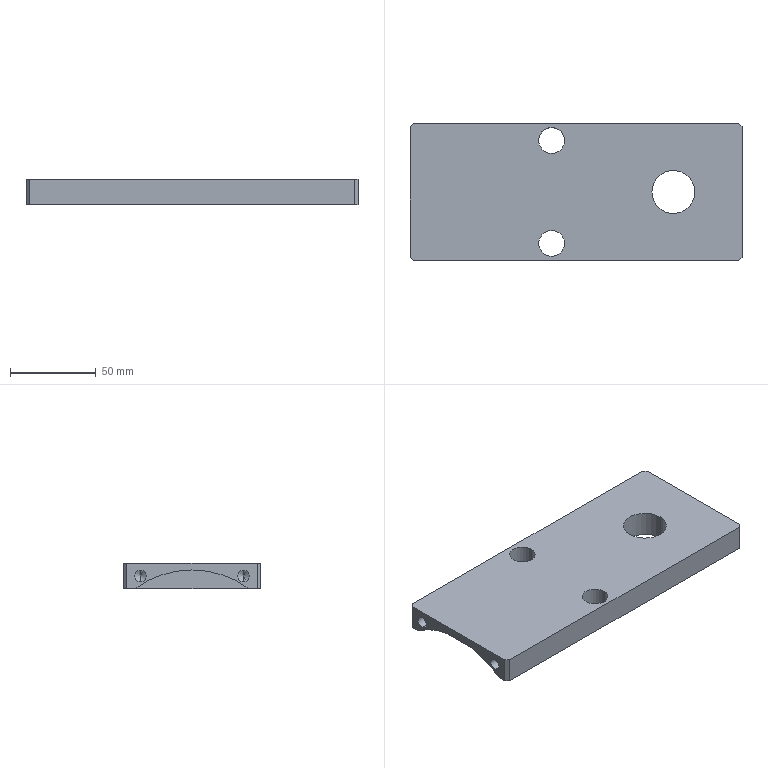Part | SolidWorks | features HoleWzd 4, Chamfer 1, Extrusion 1, ICE 1 | 1 solid | 34 faces | box 193.5 x 80 x 15 mm | volume 211454 mm3 | cylinder 15 | plane 11 | cone 8 | commonest cylinder face diameters 6.8 x8 15 x4 25 x2 112 x1
STEP:
#1=CARTESIAN_POINT('',(-77.,30.,-3.4));
#2=VERTEX_POINT('',#1);
#3=CARTESIAN_POINT('',(-77.,30.,3.4));
#4=VERTEX_POINT('',#3);
#5=CARTESIAN_POINT('',(-77.,30.,0.));
#6=DIRECTION('',(-1.,0.,0.));
#7=DIRECTION('',(0.,0.,1.));
#8=AXIS2_PLACEMENT_3D('',#5,#6,#7);
#9=CIRCLE('',#8,3.4);
#10=EDGE_CURVE('',#2,#4,#9,.T.);
#11=ORIENTED_EDGE('',*,*,#10,.F.);
#12=CARTESIAN_POINT('',(-96.75,30.,-3.4));
#13=VERTEX_POINT('',#12);
#14=CARTESIAN_POINT('',(-96.75,30.,-3.4));
#15=DIRECTION('',(-1.,0.,0.));
#16=VECTOR('',#15,1000.);
#17=LINE('',#14,#16);
#18=EDGE_CURVE('',#2,#13,#17,.T.);
#19=ORIENTED_EDGE('',*,*,#18,.T.);
#20=CARTESIAN_POINT('',(-96.75,30.,3.4));
#21=VERTEX_POINT('',#20);
#22=CARTESIAN_POINT('',(-96.75,30.,0.));
#23=DIRECTION('',(-1.,0.,0.));
#24=DIRECTION('',(0.,0.,1.));
#25=AXIS2_PLACEMENT_3D('',#22,#23,#24);
#26=CIRCLE('',#25,3.4);
#27=EDGE_CURVE('',#13,#21,#26,.T.);
#28=ORIENTED_EDGE('',*,*,#27,.T.);
#29=CARTESIAN_POINT('',(-96.75,30.,3.4));
#30=DIRECTION('',(-1.,0.,0.));
#31=VECTOR('',#30,1000.);
#32=LINE('',#29,#31);
#33=EDGE_CURVE('',#4,#21,#32,.T.);
#34=ORIENTED_EDGE('',*,*,#33,.F.);
#35=EDGE_LOOP('',(#11,#19,#28,#34));
#36=FACE_OUTER_BOUND('',#35,.T.);
#37=CARTESIAN_POINT('',(-96.75,30.,0.));
#38=DIRECTION('',(-1.,0.,0.));
#39=DIRECTION('',(0.,0.,1.));
#40=AXIS2_PLACEMENT_3D('',#37,#38,#39);
#41=CYLINDRICAL_SURFACE('',#40,3.4);
#42=ADVANCED_FACE('',(#36),#41,.F.);
#43=CARTESIAN_POINT('',(-74.957,30.,0.));
#44=VERTEX_POINT('',#43);
#45=CARTESIAN_POINT('',(-77.,30.,3.4));
#46=DIRECTION('',(-0.515,0.,0.8572));
#47=VECTOR('',#46,1000.);
#48=LINE('',#45,#47);
#49=EDGE_CURVE('',#44,#4,#48,.T.);
#50=ORIENTED_EDGE('',*,*,#49,.F.);
#51=CARTESIAN_POINT('',(-77.,30.,-3.4));
#52=DIRECTION('',(-0.515,0.,-0.8572));
#53=VECTOR('',#52,1000.);
#54=LINE('',#51,#53);
#55=EDGE_CURVE('',#44,#2,#54,.T.);
#56=ORIENTED_EDGE('',*,*,#55,.T.);
#57=ORIENTED_EDGE('',*,*,#10,.T.);
#58=EDGE_LOOP('',(#50,#56,#57));
#59=FACE_OUTER_BOUND('',#58,.T.);
#60=CARTESIAN_POINT('',(-77.,30.,0.));
#61=DIRECTION('',(-1.,0.,0.));
#62=DIRECTION('',(0.,0.,1.));
#63=AXIS2_PLACEMENT_3D('',#60,#61,#62);
#64=CONICAL_SURFACE('',#63,3.4,1.03);
#65=ADVANCED_FACE('',(#59),#64,.F.);
#66=CARTESIAN_POINT('',(-77.,-30.,-3.4));
#67=VERTEX_POINT('',#66);
#68=CARTESIAN_POINT('',(-77.,-30.,3.4));
#69=VERTEX_POINT('',#68);
#70=CARTESIAN_POINT('',(-77.,-30.,0.));
#71=DIRECTION('',(-1.,0.,0.));
#72=DIRECTION('',(0.,0.,1.));
#73=AXIS2_PLACEMENT_3D('',#70,#71,#72);
#74=CIRCLE('',#73,3.4);
#75=EDGE_CURVE('',#67,#69,#74,.T.);
#76=ORIENTED_EDGE('',*,*,#75,.F.);
#77=CARTESIAN_POINT('',(-96.75,-30.,-3.4));
#78=VERTEX_POINT('',#77);
#79=CARTESIAN_POINT('',(-96.75,-30.,-3.4));
#80=DIRECTION('',(-1.,0.,0.));
#81=VECTOR('',#80,1000.);
#82=LINE('',#79,#81);
#83=EDGE_CURVE('',#67,#78,#82,.T.);
#84=ORIENTED_EDGE('',*,*,#83,.T.);
#85=CARTESIAN_POINT('',(-96.75,-30.,3.4));
#86=VERTEX_POINT('',#85);
#87=CARTESIAN_POINT('',(-96.75,-30.,0.));
#88=DIRECTION('',(-1.,0.,0.));
#89=DIRECTION('',(0.,0.,1.));
#90=AXIS2_PLACEMENT_3D('',#87,#88,#89);
#91=CIRCLE('',#90,3.4);
#92=EDGE_CURVE('',#78,#86,#91,.T.);
#93=ORIENTED_EDGE('',*,*,#92,.T.);
#94=CARTESIAN_POINT('',(-96.75,-30.,3.4));
#95=DIRECTION('',(-1.,0.,0.));
#96=VECTOR('',#95,1000.);
#97=LINE('',#94,#96);
#98=EDGE_CURVE('',#69,#86,#97,.T.);
#99=ORIENTED_EDGE('',*,*,#98,.F.);
#100=EDGE_LOOP('',(#76,#84,#93,#99));
#101=FACE_OUTER_BOUND('',#100,.T.);
#102=CARTESIAN_POINT('',(-96.75,-30.,0.));
#103=DIRECTION('',(-1.,0.,0.));
#104=DIRECTION('',(0.,0.,1.));
#105=AXIS2_PLACEMENT_3D('',#102,#103,#104);
#106=CYLINDRICAL_SURFACE('',#105,3.4);
#107=ADVANCED_FACE('',(#101),#106,.F.);
#108=CARTESIAN_POINT('',(-74.957,-30.,0.));
#109=VERTEX_POINT('',#108);
#110=CARTESIAN_POINT('',(-77.,-30.,3.4));
#111=DIRECTION('',(-0.515,0.,0.8572));
#112=VECTOR('',#111,1000.);
#113=LINE('',#110,#112);
#114=EDGE_CURVE('',#109,#69,#113,.T.);
#115=ORIENTED_EDGE('',*,*,#114,.F.);
#116=CARTESIAN_POINT('',(-77.,-30.,-3.4));
#117=DIRECTION('',(-0.515,0.,-0.8572));
#118=VECTOR('',#117,1000.);
#119=LINE('',#116,#118);
#120=EDGE_CURVE('',#109,#67,#119,.T.);
#121=ORIENTED_EDGE('',*,*,#120,.T.);
#122=ORIENTED_EDGE('',*,*,#75,.T.);
#123=EDGE_LOOP('',(#115,#121,#122));
#124=FACE_OUTER_BOUND('',#123,.T.);
#125=CARTESIAN_POINT('',(-77.,-30.,0.));
#126=DIRECTION('',(-1.,0.,0.));
#127=DIRECTION('',(0.,0.,1.));
#128=AXIS2_PLACEMENT_3D('',#125,#126,#127);
#129=CONICAL_SURFACE('',#128,3.4,1.03);
#130=ADVANCED_FACE('',(#124),#129,.F.);
#131=CARTESIAN_POINT('',(77.,30.,3.4));
#132=VERTEX_POINT('',#131);
#133=CARTESIAN_POINT('',(77.,30.,-3.4));
#134=VERTEX_POINT('',#133);
#135=CARTESIAN_POINT('',(77.,30.,0.));
#136=DIRECTION('',(1.,0.,0.));
#137=DIRECTION('',(0.,0.,-1.));
#138=AXIS2_PLACEMENT_3D('',#135,#136,#137);
#139=CIRCLE('',#138,3.4);
#140=EDGE_CURVE('',#132,#134,#139,.T.);
#141=ORIENTED_EDGE('',*,*,#140,.F.);
#142=CARTESIAN_POINT('',(96.75,30.,3.4));
#143=VERTEX_POINT('',#142);
#144=CARTESIAN_POINT('',(96.75,30.,3.4));
#145=DIRECTION('',(1.,0.,0.));
#146=VECTOR('',#145,1000.);
#147=LINE('',#144,#146);
#148=EDGE_CURVE('',#132,#143,#147,.T.);
#149=ORIENTED_EDGE('',*,*,#148,.T.);
#150=CARTESIAN_POINT('',(96.75,30.,-3.4));
#151=VERTEX_POINT('',#150);
#152=CARTESIAN_POINT('',(96.75,30.,0.));
#153=DIRECTION('',(1.,0.,0.));
#154=DIRECTION('',(0.,0.,-1.));
#155=AXIS2_PLACEMENT_3D('',#152,#153,#154);
#156=CIRCLE('',#155,3.4);
#157=EDGE_CURVE('',#143,#151,#156,.T.);
#158=ORIENTED_EDGE('',*,*,#157,.T.);
#159=CARTESIAN_POINT('',(96.75,30.,-3.4));
#160=DIRECTION('',(1.,0.,0.));
#161=VECTOR('',#160,1000.);
#162=LINE('',#159,#161);
#163=EDGE_CURVE('',#134,#151,#162,.T.);
#164=ORIENTED_EDGE('',*,*,#163,.F.);
#165=EDGE_LOOP('',(#141,#149,#158,#164));
#166=FACE_OUTER_BOUND('',#165,.T.);
#167=CARTESIAN_POINT('',(96.75,30.,0.));
#168=DIRECTION('',(1.,0.,0.));
#169=DIRECTION('',(0.,0.,-1.));
#170=AXIS2_PLACEMENT_3D('',#167,#168,#169);
#171=CYLINDRICAL_SURFACE('',#170,3.4);
#172=ADVANCED_FACE('',(#166),#171,.F.);
#173=CARTESIAN_POINT('',(74.957,30.,0.));
#174=VERTEX_POINT('',#173);
#175=CARTESIAN_POINT('',(77.,30.,-3.4));
#176=DIRECTION('',(0.515,0.,-0.8572));
#177=VECTOR('',#176,1000.);
#178=LINE('',#175,#177);
#179=EDGE_CURVE('',#174,#134,#178,.T.);
#180=ORIENTED_EDGE('',*,*,#179,.F.);
#181=CARTESIAN_POINT('',(77.,30.,3.4));
#182=DIRECTION('',(0.515,0.,0.8572));
#183=VECTOR('',#182,1000.);
#184=LINE('',#181,#183);
#185=EDGE_CURVE('',#174,#132,#184,.T.);
#186=ORIENTED_EDGE('',*,*,#185,.T.);
#187=ORIENTED_EDGE('',*,*,#140,.T.);
#188=EDGE_LOOP('',(#180,#186,#187));
#189=FACE_OUTER_BOUND('',#188,.T.);
#190=CARTESIAN_POINT('',(77.,30.,0.));
#191=DIRECTION('',(1.,0.,0.));
#192=DIRECTION('',(0.,0.,-1.));
#193=AXIS2_PLACEMENT_3D('',#190,#191,#192);
#194=CONICAL_SURFACE('',#193,3.4,1.03);
#195=ADVANCED_FACE('',(#189),#194,.F.);
#196=CARTESIAN_POINT('',(77.,-30.,3.4));
#197=VERTEX_POINT('',#196);
#198=CARTESIAN_POINT('',(77.,-30.,-3.4));
#199=VERTEX_POINT('',#198);
#200=CARTESIAN_POINT('',(77.,-30.,0.));
#201=DIRECTION('',(1.,0.,0.));
#202=DIRECTION('',(0.,0.,-1.));
#203=AXIS2_PLACEMENT_3D('',#200,#201,#202);
#204=CIRCLE('',#203,3.4);
#205=EDGE_CURVE('',#197,#199,#204,.T.);
#206=ORIENTED_EDGE('',*,*,#205,.F.);
#207=CARTESIAN_POINT('',(96.75,-30.,3.4));
#208=VERTEX_POINT('',#207);
#209=CARTESIAN_POINT('',(96.75,-30.,3.4));
#210=DIRECTION('',(1.,0.,0.));
#211=VECTOR('',#210,1000.);
#212=LINE('',#209,#211);
#213=EDGE_CURVE('',#197,#208,#212,.T.);
#214=ORIENTED_EDGE('',*,*,#213,.T.);
#215=CARTESIAN_POINT('',(96.75,-30.,-3.4));
#216=VERTEX_POINT('',#215);
#217=CARTESIAN_POINT('',(96.75,-30.,0.));
#218=DIRECTION('',(1.,0.,0.));
#219=DIRECTION('',(0.,0.,-1.));
#220=AXIS2_PLACEMENT_3D('',#217,#218,#219);
#221=CIRCLE('',#220,3.4);
#222=EDGE_CURVE('',#208,#216,#221,.T.);
#223=ORIENTED_EDGE('',*,*,#222,.T.);
#224=CARTESIAN_POINT('',(96.75,-30.,-3.4));
#225=DIRECTION('',(1.,0.,0.));
#226=VECTOR('',#225,1000.);
#227=LINE('',#224,#226);
#228=EDGE_CURVE('',#199,#216,#227,.T.);
#229=ORIENTED_EDGE('',*,*,#228,.F.);
#230=EDGE_LOOP('',(#206,#214,#223,#229));
#231=FACE_OUTER_BOUND('',#230,.T.);
#232=CARTESIAN_POINT('',(96.75,-30.,0.));
#233=DIRECTION('',(1.,0.,0.));
#234=DIRECTION('',(0.,0.,-1.));
#235=AXIS2_PLACEMENT_3D('',#232,#233,#234);
#236=CYLINDRICAL_SURFACE('',#235,3.4);
#237=ADVANCED_FACE('',(#231),#236,.F.);
#238=CARTESIAN_POINT('',(74.957,-30.,0.));
#239=VERTEX_POINT('',#238);
#240=CARTESIAN_POINT('',(77.,-30.,-3.4));
#241=DIRECTION('',(0.515,0.,-0.8572));
#242=VECTOR('',#241,1000.);
#243=LINE('',#240,#242);
#244=EDGE_CURVE('',#239,#199,#243,.T.);
#245=ORIENTED_EDGE('',*,*,#244,.F.);
#246=CARTESIAN_POINT('',(77.,-30.,3.4));
#247=DIRECTION('',(0.515,0.,0.8572));
#248=VECTOR('',#247,1000.);
#249=LINE('',#246,#248);
#250=EDGE_CURVE('',#239,#197,#249,.T.);
#251=ORIENTED_EDGE('',*,*,#250,.T.);
#252=ORIENTED_EDGE('',*,*,#205,.T.);
#253=EDGE_LOOP('',(#245,#251,#252));
#254=FACE_OUTER_BOUND('',#253,.T.);
#255=CARTESIAN_POINT('',(77.,-30.,0.));
#256=DIRECTION('',(1.,0.,0.));
#257=DIRECTION('',(0.,0.,-1.));
#258=AXIS2_PLACEMENT_3D('',#255,#256,#257);
#259=CONICAL_SURFACE('',#258,3.4,1.03);
#260=ADVANCED_FACE('',(#254),#259,.F.);
#261=CARTESIAN_POINT('',(-21.75,30.,-7.5));
#262=VERTEX_POINT('',#261);
#263=CARTESIAN_POINT('',(-6.75,30.,-7.5));
#264=VERTEX_POINT('',#263);
#265=CARTESIAN_POINT('',(-14.25,30.,-7.5));
#266=DIRECTION('',(0.,0.,1.));
#267=DIRECTION('',(1.,0.,0.));
#268=AXIS2_PLACEMENT_3D('',#265,#266,#267);
#269=CIRCLE('',#268,7.5);
#270=EDGE_CURVE('',#262,#264,#269,.T.);
#271=ORIENTED_EDGE('',*,*,#270,.F.);
#272=CARTESIAN_POINT('',(-21.75,30.,7.5));
#273=VERTEX_POINT('',#272);
#274=CARTESIAN_POINT('',(-21.75,30.,7.5));
#275=DIRECTION('',(0.,0.,1.));
#276=VECTOR('',#275,1000.);
#277=LINE('',#274,#276);
#278=EDGE_CURVE('',#262,#273,#277,.T.);
#279=ORIENTED_EDGE('',*,*,#278,.T.);
#280=CARTESIAN_POINT('',(-6.75,30.,7.5));
#281=VERTEX_POINT('',#280);
#282=CARTESIAN_POINT('',(-14.25,30.,7.5));
#283=DIRECTION('',(0.,0.,1.));
#284=DIRECTION('',(1.,0.,0.));
#285=AXIS2_PLACEMENT_3D('',#282,#283,#284);
#286=CIRCLE('',#285,7.5);
#287=EDGE_CURVE('',#273,#281,#286,.T.);
#288=ORIENTED_EDGE('',*,*,#287,.T.);
#289=CARTESIAN_POINT('',(-6.75,30.,7.5));
#290=DIRECTION('',(0.,0.,1.));
#291=VECTOR('',#290,1000.);
#292=LINE('',#289,#291);
#293=EDGE_CURVE('',#264,#281,#292,.T.);
#294=ORIENTED_EDGE('',*,*,#293,.F.);
#295=EDGE_LOOP('',(#271,#279,#288,#294));
#296=FACE_OUTER_BOUND('',#295,.T.);
#297=CARTESIAN_POINT('',(-14.25,30.,7.5));
#298=DIRECTION('',(0.,0.,1.));
#299=DIRECTION('',(1.,0.,0.));
#300=AXIS2_PLACEMENT_3D('',#297,#298,#299);
#301=CYLINDRICAL_SURFACE('',#300,7.5);
#302=ADVANCED_FACE('',(#296),#301,.F.);
#303=CARTESIAN_POINT('',(-21.75,-30.,-7.5));
#304=VERTEX_POINT('',#303);
#305=CARTESIAN_POINT('',(-6.75,-30.,-7.5));
#306=VERTEX_POINT('',#305);
#307=CARTESIAN_POINT('',(-14.25,-30.,-7.5));
#308=DIRECTION('',(0.,0.,1.));
#309=DIRECTION('',(1.,0.,0.));
#310=AXIS2_PLACEMENT_3D('',#307,#308,#309);
#311=CIRCLE('',#310,7.5);
#312=EDGE_CURVE('',#304,#306,#311,.T.);
#313=ORIENTED_EDGE('',*,*,#312,.F.);
#314=CARTESIAN_POINT('',(-21.75,-30.,7.5));
#315=VERTEX_POINT('',#314);
#316=CARTESIAN_POINT('',(-21.75,-30.,7.5));
#317=DIRECTION('',(0.,0.,1.));
#318=VECTOR('',#317,1000.);
#319=LINE('',#316,#318);
#320=EDGE_CURVE('',#304,#315,#319,.T.);
#321=ORIENTED_EDGE('',*,*,#320,.T.);
#322=CARTESIAN_POINT('',(-6.75,-30.,7.5));
#323=VERTEX_POINT('',#322);
#324=CARTESIAN_POINT('',(-14.25,-30.,7.5));
#325=DIRECTION('',(0.,0.,1.));
#326=DIRECTION('',(1.,0.,0.));
#327=AXIS2_PLACEMENT_3D('',#324,#325,#326);
#328=CIRCLE('',#327,7.5);
#329=EDGE_CURVE('',#315,#323,#328,.T.);
#330=ORIENTED_EDGE('',*,*,#329,.T.);
#331=CARTESIAN_POINT('',(-6.75,-30.,7.5));
#332=DIRECTION('',(0.,0.,1.));
#333=VECTOR('',#332,1000.);
#334=LINE('',#331,#333);
#335=EDGE_CURVE('',#306,#323,#334,.T.);
#336=ORIENTED_EDGE('',*,*,#335,.F.);
#337=EDGE_LOOP('',(#313,#321,#330,#336));
#338=FACE_OUTER_BOUND('',#337,.T.);
#339=CARTESIAN_POINT('',(-14.25,-30.,7.5));
#340=DIRECTION('',(0.,0.,1.));
#341=DIRECTION('',(1.,0.,0.));
#342=AXIS2_PLACEMENT_3D('',#339,#340,#341);
#343=CYLINDRICAL_SURFACE('',#342,7.5);
#344=ADVANCED_FACE('',(#338),#343,.F.);
#345=CARTESIAN_POINT('',(44.25,0.,-7.5));
#346=VERTEX_POINT('',#345);
#347=CARTESIAN_POINT('',(69.25,0.,-7.5));
#348=VERTEX_POINT('',#347);
#349=CARTESIAN_POINT('',(56.75,0.,-7.5));
#350=DIRECTION('',(0.,0.,1.));
#351=DIRECTION('',(1.,0.,0.));
#352=AXIS2_PLACEMENT_3D('',#349,#350,#351);
#353=CIRCLE('',#352,12.5);
#354=EDGE_CURVE('',#346,#348,#353,.T.);
#355=ORIENTED_EDGE('',*,*,#354,.F.);
#356=CARTESIAN_POINT('',(44.25,0.,7.5));
#357=VERTEX_POINT('',#356);
#358=CARTESIAN_POINT('',(44.25,0.,7.5));
#359=DIRECTION('',(0.,0.,1.));
#360=VECTOR('',#359,1000.);
#361=LINE('',#358,#360);
#362=EDGE_CURVE('',#346,#357,#361,.T.);
#363=ORIENTED_EDGE('',*,*,#362,.T.);
#364=CARTESIAN_POINT('',(69.25,0.,7.5));
#365=VERTEX_POINT('',#364);
#366=CARTESIAN_POINT('',(56.75,0.,7.5));
#367=DIRECTION('',(0.,0.,1.));
#368=DIRECTION('',(1.,0.,0.));
#369=AXIS2_PLACEMENT_3D('',#366,#367,#368);
#370=CIRCLE('',#369,12.5);
#371=EDGE_CURVE('',#357,#365,#370,.T.);
#372=ORIENTED_EDGE('',*,*,#371,.T.);
#373=CARTESIAN_POINT('',(69.25,0.,7.5));
#374=DIRECTION('',(0.,0.,1.));
#375=VECTOR('',#374,1000.);
#376=LINE('',#373,#375);
#377=EDGE_CURVE('',#348,#365,#376,.T.);
#378=ORIENTED_EDGE('',*,*,#377,.F.);
#379=EDGE_LOOP('',(#355,#363,#372,#378));
#380=FACE_OUTER_BOUND('',#379,.T.);
#381=CARTESIAN_POINT('',(56.75,0.,7.5));
#382=DIRECTION('',(0.,0.,1.));
#383=DIRECTION('',(1.,0.,0.));
#384=AXIS2_PLACEMENT_3D('',#381,#382,#383);
#385=CYLINDRICAL_SURFACE('',#384,12.5);
#386=ADVANCED_FACE('',(#380),#385,.F.);
#387=CARTESIAN_POINT('',(96.75,30.,0.));
#388=DIRECTION('',(1.,0.,0.));
#389=DIRECTION('',(0.,0.,-1.));
#390=AXIS2_PLACEMENT_3D('',#387,#388,#389);
#391=CIRCLE('',#390,3.4);
#392=EDGE_CURVE('',#151,#143,#391,.T.);
#393=ORIENTED_EDGE('',*,*,#392,.F.);
#394=ORIENTED_EDGE('',*,*,#157,.F.);
#395=EDGE_LOOP('',(#393,#394));
#396=FACE_BOUND('',#395,.T.);
#397=CARTESIAN_POINT('',(96.75,-30.,0.));
#398=DIRECTION('',(1.,0.,0.));
#399=DIRECTION('',(0.,0.,-1.));
#400=AXIS2_PLACEMENT_3D('',#397,#398,#399);
#401=CIRCLE('',#400,3.4);
#402=EDGE_CURVE('',#216,#208,#401,.T.);
#403=ORIENTED_EDGE('',*,*,#402,.F.);
#404=ORIENTED_EDGE('',*,*,#222,.F.);
#405=EDGE_LOOP('',(#403,#404));
#406=FACE_BOUND('',#405,.T.);
#407=CARTESIAN_POINT('',(96.75,-38.,7.5));
#408=VERTEX_POINT('',#407);
#409=CARTESIAN_POINT('',(96.75,38.,7.5));
#410=VERTEX_POINT('',#409);
#411=CARTESIAN_POINT('',(96.75,40.,7.5));
#412=DIRECTION('',(0.,1.,0.));
#413=VECTOR('',#412,1000.);
#414=LINE('',#411,#413);
#415=EDGE_CURVE('',#408,#410,#414,.T.);
#416=ORIENTED_EDGE('',*,*,#415,.F.);
#417=CARTESIAN_POINT('',(96.75,-38.,-7.5));
#418=VERTEX_POINT('',#417);
#419=CARTESIAN_POINT('',(96.75,-38.,7.5));
#420=DIRECTION('',(0.,0.,-1.));
#421=VECTOR('',#420,1000.);
#422=LINE('',#419,#421);
#423=EDGE_CURVE('',#408,#418,#422,.T.);
#424=ORIENTED_EDGE('',*,*,#423,.T.);
#425=CARTESIAN_POINT('',(96.75,38.,-7.5));
#426=VERTEX_POINT('',#425);
#427=CARTESIAN_POINT('',(96.75,40.,-7.5));
#428=DIRECTION('',(0.,1.,0.));
#429=VECTOR('',#428,1000.);
#430=LINE('',#427,#429);
#431=EDGE_CURVE('',#418,#426,#430,.T.);
#432=ORIENTED_EDGE('',*,*,#431,.T.);
#433=CARTESIAN_POINT('',(96.75,38.,7.5));
#434=DIRECTION('',(0.,0.,1.));
#435=VECTOR('',#434,1000.);
#436=LINE('',#433,#435);
#437=EDGE_CURVE('',#426,#410,#436,.T.);
#438=ORIENTED_EDGE('',*,*,#437,.T.);
#439=EDGE_LOOP('',(#416,#424,#432,#438));
#440=FACE_OUTER_BOUND('',#439,.T.);
#441=CARTESIAN_POINT('',(96.75,40.,7.5));
#442=DIRECTION('',(-1.,0.,0.));
#443=DIRECTION('',(0.,0.,1.));
#444=AXIS2_PLACEMENT_3D('',#441,#442,#443);
#445=PLANE('',#444);
#446=ADVANCED_FACE('',(#396,#406,#440),#445,.F.);
#447=CARTESIAN_POINT('',(94.75,40.,-7.5));
#448=VERTEX_POINT('',#447);
#449=CARTESIAN_POINT('',(-94.75,40.,-7.5));
#450=VERTEX_POINT('',#449);
#451=CARTESIAN_POINT('',(-96.75,40.,-7.5));
#452=DIRECTION('',(-1.,0.,0.));
#453=VECTOR('',#452,1000.);
#454=LINE('',#451,#453);
#455=EDGE_CURVE('',#448,#450,#454,.T.);
#456=ORIENTED_EDGE('',*,*,#455,.T.);
#457=CARTESIAN_POINT('',(-94.75,40.,7.5));
#458=VERTEX_POINT('',#457);
#459=CARTESIAN_POINT('',(-94.75,40.,7.5));
#460=DIRECTION('',(0.,0.,1.));
#461=VECTOR('',#460,1000.);
#462=LINE('',#459,#461);
#463=EDGE_CURVE('',#450,#458,#462,.T.);
#464=ORIENTED_EDGE('',*,*,#463,.T.);
#465=CARTESIAN_POINT('',(94.75,40.,7.5));
#466=VERTEX_POINT('',#465);
#467=CARTESIAN_POINT('',(-96.75,40.,7.5));
#468=DIRECTION('',(-1.,0.,0.));
#469=VECTOR('',#468,1000.);
#470=LINE('',#467,#469);
#471=EDGE_CURVE('',#466,#458,#470,.T.);
#472=ORIENTED_EDGE('',*,*,#471,.F.);
#473=CARTESIAN_POINT('',(94.75,40.,7.5));
#474=DIRECTION('',(0.,0.,-1.));
#475=VECTOR('',#474,1000.);
#476=LINE('',#473,#475);
#477=EDGE_CURVE('',#466,#448,#476,.T.);
#478=ORIENTED_EDGE('',*,*,#477,.T.);
#479=EDGE_LOOP('',(#456,#464,#472,#478));
#480=FACE_OUTER_BOUND('',#479,.T.);
#481=CARTESIAN_POINT('',(-96.75,40.,7.5));
#482=DIRECTION('',(0.,-1.,0.));
#483=DIRECTION('',(0.,0.,-1.));
#484=AXIS2_PLACEMENT_3D('',#481,#482,#483);
#485=PLANE('',#484);
#486=ADVANCED_FACE('',(#480),#485,.F.);
#487=CARTESIAN_POINT('',(-96.75,30.,0.));
#488=DIRECTION('',(-1.,0.,0.));
#489=DIRECTION('',(0.,0.,1.));
#490=AXIS2_PLACEMENT_3D('',#487,#488,#489);
#491=CIRCLE('',#490,3.4);
#492=EDGE_CURVE('',#21,#13,#491,.T.);
#493=ORIENTED_EDGE('',*,*,#492,.F.);
#494=ORIENTED_EDGE('',*,*,#27,.F.);
#495=EDGE_LOOP('',(#493,#494));
#496=FACE_BOUND('',#495,.T.);
#497=CARTESIAN_POINT('',(-96.75,-30.,0.));
#498=DIRECTION('',(-1.,0.,0.));
#499=DIRECTION('',(0.,0.,1.));
#500=AXIS2_PLACEMENT_3D('',#497,#498,#499);
#501=CIRCLE('',#500,3.4);
#502=EDGE_CURVE('',#86,#78,#501,.T.);
#503=ORIENTED_EDGE('',*,*,#502,.F.);
#504=ORIENTED_EDGE('',*,*,#92,.F.);
#505=EDGE_LOOP('',(#503,#504));
#506=FACE_BOUND('',#505,.T.);
#507=CARTESIAN_POINT('',(-96.75,38.,7.5));
#508=VERTEX_POINT('',#507);
#509=CARTESIAN_POINT('',(-96.75,-38.,7.5));
#510=VERTEX_POINT('',#509);
#511=CARTESIAN_POINT('',(-96.75,40.,7.5));
#512=DIRECTION('',(0.,-1.,0.));
#513=VECTOR('',#512,1000.);
#514=LINE('',#511,#513);
#515=EDGE_CURVE('',#508,#510,#514,.T.);
#516=ORIENTED_EDGE('',*,*,#515,.F.);
#517=CARTESIAN_POINT('',(-96.75,38.,-7.5));
#518=VERTEX_POINT('',#517);
#519=CARTESIAN_POINT('',(-96.75,38.,7.5));
#520=DIRECTION('',(0.,0.,-1.));
#521=VECTOR('',#520,1000.);
#522=LINE('',#519,#521);
#523=EDGE_CURVE('',#508,#518,#522,.T.);
#524=ORIENTED_EDGE('',*,*,#523,.T.);
#525=CARTESIAN_POINT('',(-96.75,33.332,-7.5));
#526=VERTEX_POINT('',#525);
#527=CARTESIAN_POINT('',(-96.75,40.,-7.5));
#528=DIRECTION('',(0.,-1.,0.));
#529=VECTOR('',#528,1000.);
#530=LINE('',#527,#529);
#531=EDGE_CURVE('',#518,#526,#530,.T.);
#532=ORIENTED_EDGE('',*,*,#531,.T.);
#533=CARTESIAN_POINT('',(-96.75,-33.332,-7.5));
#534=VERTEX_POINT('',#533);
#535=CARTESIAN_POINT('',(-96.75,0.,-52.5));
#536=DIRECTION('',(-1.,0.,0.));
#537=DIRECTION('',(0.,-1.,0.));
#538=AXIS2_PLACEMENT_3D('',#535,#536,#537);
#539=CIRCLE('',#538,56.);
#540=EDGE_CURVE('',#534,#526,#539,.T.);
#541=ORIENTED_EDGE('',*,*,#540,.F.);
#542=CARTESIAN_POINT('',(-96.75,-38.,-7.5));
#543=VERTEX_POINT('',#542);
#544=CARTESIAN_POINT('',(-96.75,40.,-7.5));
#545=DIRECTION('',(0.,-1.,0.));
#546=VECTOR('',#545,1000.);
#547=LINE('',#544,#546);
#548=EDGE_CURVE('',#534,#543,#547,.T.);
#549=ORIENTED_EDGE('',*,*,#548,.T.);
#550=CARTESIAN_POINT('',(-96.75,-38.,7.5));
#551=DIRECTION('',(0.,0.,1.));
#552=VECTOR('',#551,1000.);
#553=LINE('',#550,#552);
#554=EDGE_CURVE('',#543,#510,#553,.T.);
#555=ORIENTED_EDGE('',*,*,#554,.T.);
#556=EDGE_LOOP('',(#516,#524,#532,#541,#549,#555));
#557=FACE_OUTER_BOUND('',#556,.T.);
#558=CARTESIAN_POINT('',(-96.75,40.,7.5));
#559=DIRECTION('',(1.,0.,0.));
#560=DIRECTION('',(0.,0.,-1.));
#561=AXIS2_PLACEMENT_3D('',#558,#559,#560);
#562=PLANE('',#561);
#563=ADVANCED_FACE('',(#496,#506,#557),#562,.F.);
#564=CARTESIAN_POINT('',(-94.75,-40.,7.5));
#565=VERTEX_POINT('',#564);
#566=CARTESIAN_POINT('',(94.75,-40.,7.5));
#567=VERTEX_POINT('',#566);
#568=CARTESIAN_POINT('',(-96.75,-40.,7.5));
#569=DIRECTION('',(1.,0.,0.));
#570=VECTOR('',#569,1000.);
#571=LINE('',#568,#570);
#572=EDGE_CURVE('',#565,#567,#571,.T.);
#573=ORIENTED_EDGE('',*,*,#572,.F.);
#574=CARTESIAN_POINT('',(-94.75,-40.,-7.5));
#575=VERTEX_POINT('',#574);
#576=CARTESIAN_POINT('',(-94.75,-40.,7.5));
#577=DIRECTION('',(0.,0.,-1.));
#578=VECTOR('',#577,1000.);
#579=LINE('',#576,#578);
#580=EDGE_CURVE('',#565,#575,#579,.T.);
#581=ORIENTED_EDGE('',*,*,#580,.T.);
#582=CARTESIAN_POINT('',(94.75,-40.,-7.5));
#583=VERTEX_POINT('',#582);
#584=CARTESIAN_POINT('',(-96.75,-40.,-7.5));
#585=DIRECTION('',(1.,0.,0.));
#586=VECTOR('',#585,1000.);
#587=LINE('',#584,#586);
#588=EDGE_CURVE('',#575,#583,#587,.T.);
#589=ORIENTED_EDGE('',*,*,#588,.T.);
#590=CARTESIAN_POINT('',(94.75,-40.,7.5));
#591=DIRECTION('',(0.,0.,1.));
#592=VECTOR('',#591,1000.);
#593=LINE('',#590,#592);
#594=EDGE_CURVE('',#583,#567,#593,.T.);
#595=ORIENTED_EDGE('',*,*,#594,.T.);
#596=EDGE_LOOP('',(#573,#581,#589,#595));
#597=FACE_OUTER_BOUND('',#596,.T.);
#598=CARTESIAN_POINT('',(-96.75,-40.,7.5));
#599=DIRECTION('',(0.,1.,0.));
#600=DIRECTION('',(0.,0.,1.));
#601=AXIS2_PLACEMENT_3D('',#598,#599,#600);
#602=PLANE('',#601);
#603=ADVANCED_FACE('',(#597),#602,.F.);
#604=CARTESIAN_POINT('',(-14.25,30.,7.5));
#605=DIRECTION('',(0.,0.,1.));
#606=DIRECTION('',(1.,0.,0.));
#607=AXIS2_PLACEMENT_3D('',#604,#605,#606);
#608=CIRCLE('',#607,7.5);
#609=EDGE_CURVE('',#281,#273,#608,.T.);
#610=ORIENTED_EDGE('',*,*,#609,.F.);
#611=ORIENTED_EDGE('',*,*,#287,.F.);
#612=EDGE_LOOP('',(#610,#611));
#613=FACE_BOUND('',#612,.T.);
#614=CARTESIAN_POINT('',(-14.25,-30.,7.5));
#615=DIRECTION('',(0.,0.,1.));
#616=DIRECTION('',(1.,0.,0.));
#617=AXIS2_PLACEMENT_3D('',#614,#615,#616);
#618=CIRCLE('',#617,7.5);
#619=EDGE_CURVE('',#323,#315,#618,.T.);
#620=ORIENTED_EDGE('',*,*,#619,.F.);
#621=ORIENTED_EDGE('',*,*,#329,.F.);
#622=EDGE_LOOP('',(#620,#621));
#623=FACE_BOUND('',#622,.T.);
#624=CARTESIAN_POINT('',(56.75,0.,7.5));
#625=DIRECTION('',(0.,0.,1.));
#626=DIRECTION('',(1.,0.,0.));
#627=AXIS2_PLACEMENT_3D('',#624,#625,#626);
#628=CIRCLE('',#627,12.5);
#629=EDGE_CURVE('',#365,#357,#628,.T.);
#630=ORIENTED_EDGE('',*,*,#629,.F.);
#631=ORIENTED_EDGE('',*,*,#371,.F.);
#632=EDGE_LOOP('',(#630,#631));
#633=FACE_BOUND('',#632,.T.);
#634=ORIENTED_EDGE('',*,*,#471,.T.);
#635=CARTESIAN_POINT('',(-67.375,67.375,7.5));
#636=DIRECTION('',(-0.7071,-0.7071,0.));
#637=VECTOR('',#636,1000.);
#638=LINE('',#635,#637);
#639=EDGE_CURVE('',#458,#508,#638,.T.);
#640=ORIENTED_EDGE('',*,*,#639,.T.);
#641=ORIENTED_EDGE('',*,*,#515,.T.);
#642=CARTESIAN_POINT('',(-67.375,-67.375,7.5));
#643=DIRECTION('',(0.7071,-0.7071,0.));
#644=VECTOR('',#643,1000.);
#645=LINE('',#642,#644);
#646=EDGE_CURVE('',#510,#565,#645,.T.);
#647=ORIENTED_EDGE('',*,*,#646,.T.);
#648=ORIENTED_EDGE('',*,*,#572,.T.);
#649=CARTESIAN_POINT('',(67.375,-67.375,7.5));
#650=DIRECTION('',(0.7071,0.7071,0.));
#651=VECTOR('',#650,1000.);
#652=LINE('',#649,#651);
#653=EDGE_CURVE('',#567,#408,#652,.T.);
#654=ORIENTED_EDGE('',*,*,#653,.T.);
#655=ORIENTED_EDGE('',*,*,#415,.T.);
#656=CARTESIAN_POINT('',(67.375,67.375,7.5));
#657=DIRECTION('',(-0.7071,0.7071,0.));
#658=VECTOR('',#657,1000.);
#659=LINE('',#656,#658);
#660=EDGE_CURVE('',#410,#466,#659,.T.);
#661=ORIENTED_EDGE('',*,*,#660,.T.);
#662=EDGE_LOOP('',(#634,#640,#641,#647,#648,#654,#655,#661));
#663=FACE_OUTER_BOUND('',#662,.T.);
#664=CARTESIAN_POINT('',(0.,0.,7.5));
#665=DIRECTION('',(0.,0.,1.));
#666=DIRECTION('',(1.,0.,0.));
#667=AXIS2_PLACEMENT_3D('',#664,#665,#666);
#668=PLANE('',#667);
#669=ADVANCED_FACE('',(#613,#623,#633,#663),#668,.T.);
#670=CARTESIAN_POINT('',(-14.25,30.,-7.5));
#671=DIRECTION('',(0.,0.,1.));
#672=DIRECTION('',(1.,0.,0.));
#673=AXIS2_PLACEMENT_3D('',#670,#671,#672);
#674=CIRCLE('',#673,7.5);
#675=EDGE_CURVE('',#264,#262,#674,.T.);
#676=ORIENTED_EDGE('',*,*,#675,.T.);
#677=ORIENTED_EDGE('',*,*,#270,.T.);
#678=EDGE_LOOP('',(#676,#677));
#679=FACE_BOUND('',#678,.T.);
#680=CARTESIAN_POINT('',(-14.25,-30.,-7.5));
#681=DIRECTION('',(0.,0.,1.));
#682=DIRECTION('',(1.,0.,0.));
#683=AXIS2_PLACEMENT_3D('',#680,#681,#682);
#684=CIRCLE('',#683,7.5);
#685=EDGE_CURVE('',#306,#304,#684,.T.);
#686=ORIENTED_EDGE('',*,*,#685,.T.);
#687=ORIENTED_EDGE('',*,*,#312,.T.);
#688=EDGE_LOOP('',(#686,#687));
#689=FACE_BOUND('',#688,.T.);
#690=CARTESIAN_POINT('',(56.75,0.,-7.5));
#691=DIRECTION('',(0.,0.,1.));
#692=DIRECTION('',(1.,0.,0.));
#693=AXIS2_PLACEMENT_3D('',#690,#691,#692);
#694=CIRCLE('',#693,12.5);
#695=EDGE_CURVE('',#348,#346,#694,.T.);
#696=ORIENTED_EDGE('',*,*,#695,.T.);
#697=ORIENTED_EDGE('',*,*,#354,.T.);
#698=EDGE_LOOP('',(#696,#697));
#699=FACE_BOUND('',#698,.T.);
#700=ORIENTED_EDGE('',*,*,#531,.F.);
#701=CARTESIAN_POINT('',(-96.75,38.,-7.5));
#702=DIRECTION('',(0.7071,0.7071,0.));
#703=VECTOR('',#702,1000.);
#704=LINE('',#701,#703);
#705=EDGE_CURVE('',#518,#450,#704,.T.);
#706=ORIENTED_EDGE('',*,*,#705,.T.);
#707=ORIENTED_EDGE('',*,*,#455,.F.);
#708=CARTESIAN_POINT('',(94.75,40.,-7.5));
#709=DIRECTION('',(0.7071,-0.7071,0.));
#710=VECTOR('',#709,1000.);
#711=LINE('',#708,#710);
#712=EDGE_CURVE('',#448,#426,#711,.T.);
#713=ORIENTED_EDGE('',*,*,#712,.T.);
#714=ORIENTED_EDGE('',*,*,#431,.F.);
#715=CARTESIAN_POINT('',(96.75,-38.,-7.5));
#716=DIRECTION('',(-0.7071,-0.7071,0.));
#717=VECTOR('',#716,1000.);
#718=LINE('',#715,#717);
#719=EDGE_CURVE('',#418,#583,#718,.T.);
#720=ORIENTED_EDGE('',*,*,#719,.T.);
#721=ORIENTED_EDGE('',*,*,#588,.F.);
#722=CARTESIAN_POINT('',(-94.75,-40.,-7.5));
#723=DIRECTION('',(-0.7071,0.7071,0.));
#724=VECTOR('',#723,1000.);
#725=LINE('',#722,#724);
#726=EDGE_CURVE('',#575,#543,#725,.T.);
#727=ORIENTED_EDGE('',*,*,#726,.T.);
#728=ORIENTED_EDGE('',*,*,#548,.F.);
#729=CARTESIAN_POINT('',(-86.75,-33.332,-7.5));
#730=VERTEX_POINT('',#729);
#731=CARTESIAN_POINT('',(-86.75,-33.332,-7.5));
#732=DIRECTION('',(1.,0.,0.));
#733=VECTOR('',#732,1000.);
#734=LINE('',#731,#733);
#735=EDGE_CURVE('',#534,#730,#734,.T.);
#736=ORIENTED_EDGE('',*,*,#735,.T.);
#737=CARTESIAN_POINT('',(-86.75,33.332,-7.5));
#738=VERTEX_POINT('',#737);
#739=CARTESIAN_POINT('',(-86.75,0.,-7.5));
#740=DIRECTION('',(0.,-1.,0.));
#741=VECTOR('',#740,1000.);
#742=LINE('',#739,#741);
#743=EDGE_CURVE('',#738,#730,#742,.T.);
#744=ORIENTED_EDGE('',*,*,#743,.F.);
#745=CARTESIAN_POINT('',(-86.75,33.332,-7.5));
#746=DIRECTION('',(-1.,0.,0.));
#747=VECTOR('',#746,1000.);
#748=LINE('',#745,#747);
#749=EDGE_CURVE('',#738,#526,#748,.T.);
#750=ORIENTED_EDGE('',*,*,#749,.T.);
#751=EDGE_LOOP('',(#700,#706,#707,#713,#714,#720,#721,#727,#728,#736,#744,#750));
#752=FACE_OUTER_BOUND('',#751,.T.);
#753=CARTESIAN_POINT('',(0.,0.,-7.5));
#754=DIRECTION('',(0.,0.,1.));
#755=DIRECTION('',(1.,0.,0.));
#756=AXIS2_PLACEMENT_3D('',#753,#754,#755);
#757=PLANE('',#756);
#758=ADVANCED_FACE('',(#679,#689,#699,#752),#757,.F.);
#759=ORIENTED_EDGE('',*,*,#362,.F.);
#760=ORIENTED_EDGE('',*,*,#695,.F.);
#761=ORIENTED_EDGE('',*,*,#377,.T.);
#762=ORIENTED_EDGE('',*,*,#629,.T.);
#763=EDGE_LOOP('',(#759,#760,#761,#762));
#764=FACE_OUTER_BOUND('',#763,.T.);
#765=CARTESIAN_POINT('',(56.75,0.,7.5));
#766=DIRECTION('',(0.,0.,1.));
#767=DIRECTION('',(1.,0.,0.));
#768=AXIS2_PLACEMENT_3D('',#765,#766,#767);
#769=CYLINDRICAL_SURFACE('',#768,12.5);
#770=ADVANCED_FACE('',(#764),#769,.F.);
#771=ORIENTED_EDGE('',*,*,#320,.F.);
#772=ORIENTED_EDGE('',*,*,#685,.F.);
#773=ORIENTED_EDGE('',*,*,#335,.T.);
#774=ORIENTED_EDGE('',*,*,#619,.T.);
#775=EDGE_LOOP('',(#771,#772,#773,#774));
#776=FACE_OUTER_BOUND('',#775,.T.);
#777=CARTESIAN_POINT('',(-14.25,-30.,7.5));
#778=DIRECTION('',(0.,0.,1.));
#779=DIRECTION('',(1.,0.,0.));
#780=AXIS2_PLACEMENT_3D('',#777,#778,#779);
#781=CYLINDRICAL_SURFACE('',#780,7.5);
#782=ADVANCED_FACE('',(#776),#781,.F.);
#783=ORIENTED_EDGE('',*,*,#278,.F.);
#784=ORIENTED_EDGE('',*,*,#675,.F.);
#785=ORIENTED_EDGE('',*,*,#293,.T.);
#786=ORIENTED_EDGE('',*,*,#609,.T.);
#787=EDGE_LOOP('',(#783,#784,#785,#786));
#788=FACE_OUTER_BOUND('',#787,.T.);
#789=CARTESIAN_POINT('',(-14.25,30.,7.5));
#790=DIRECTION('',(0.,0.,1.));
#791=DIRECTION('',(1.,0.,0.));
#792=AXIS2_PLACEMENT_3D('',#789,#790,#791);
#793=CYLINDRICAL_SURFACE('',#792,7.5);
#794=ADVANCED_FACE('',(#788),#793,.F.);
#795=ORIENTED_EDGE('',*,*,#250,.F.);
#796=ORIENTED_EDGE('',*,*,#244,.T.);
#797=CARTESIAN_POINT('',(77.,-30.,0.));
#798=DIRECTION('',(1.,0.,0.));
#799=DIRECTION('',(0.,0.,-1.));
#800=AXIS2_PLACEMENT_3D('',#797,#798,#799);
#801=CIRCLE('',#800,3.4);
#802=EDGE_CURVE('',#199,#197,#801,.T.);
#803=ORIENTED_EDGE('',*,*,#802,.T.);
#804=EDGE_LOOP('',(#795,#796,#803));
#805=FACE_OUTER_BOUND('',#804,.T.);
#806=CARTESIAN_POINT('',(77.,-30.,0.));
#807=DIRECTION('',(1.,0.,0.));
#808=DIRECTION('',(0.,0.,-1.));
#809=AXIS2_PLACEMENT_3D('',#806,#807,#808);
#810=CONICAL_SURFACE('',#809,3.4,1.03);
#811=ADVANCED_FACE('',(#805),#810,.F.);
#812=ORIENTED_EDGE('',*,*,#213,.F.);
#813=ORIENTED_EDGE('',*,*,#802,.F.);
#814=ORIENTED_EDGE('',*,*,#228,.T.);
#815=ORIENTED_EDGE('',*,*,#402,.T.);
#816=EDGE_LOOP('',(#812,#813,#814,#815));
#817=FACE_OUTER_BOUND('',#816,.T.);
#818=CARTESIAN_POINT('',(96.75,-30.,0.));
#819=DIRECTION('',(1.,0.,0.));
#820=DIRECTION('',(0.,0.,-1.));
#821=AXIS2_PLACEMENT_3D('',#818,#819,#820);
#822=CYLINDRICAL_SURFACE('',#821,3.4);
#823=ADVANCED_FACE('',(#817),#822,.F.);
#824=ORIENTED_EDGE('',*,*,#185,.F.);
#825=ORIENTED_EDGE('',*,*,#179,.T.);
#826=CARTESIAN_POINT('',(77.,30.,0.));
#827=DIRECTION('',(1.,0.,0.));
#828=DIRECTION('',(0.,0.,-1.));
#829=AXIS2_PLACEMENT_3D('',#826,#827,#828);
#830=CIRCLE('',#829,3.4);
#831=EDGE_CURVE('',#134,#132,#830,.T.);
#832=ORIENTED_EDGE('',*,*,#831,.T.);
#833=EDGE_LOOP('',(#824,#825,#832));
#834=FACE_OUTER_BOUND('',#833,.T.);
#835=CARTESIAN_POINT('',(77.,30.,0.));
#836=DIRECTION('',(1.,0.,0.));
#837=DIRECTION('',(0.,0.,-1.));
#838=AXIS2_PLACEMENT_3D('',#835,#836,#837);
#839=CONICAL_SURFACE('',#838,3.4,1.03);
#840=ADVANCED_FACE('',(#834),#839,.F.);
#841=ORIENTED_EDGE('',*,*,#148,.F.);
#842=ORIENTED_EDGE('',*,*,#831,.F.);
#843=ORIENTED_EDGE('',*,*,#163,.T.);
#844=ORIENTED_EDGE('',*,*,#392,.T.);
#845=EDGE_LOOP('',(#841,#842,#843,#844));
#846=FACE_OUTER_BOUND('',#845,.T.);
#847=CARTESIAN_POINT('',(96.75,30.,0.));
#848=DIRECTION('',(1.,0.,0.));
#849=DIRECTION('',(0.,0.,-1.));
#850=AXIS2_PLACEMENT_3D('',#847,#848,#849);
#851=CYLINDRICAL_SURFACE('',#850,3.4);
#852=ADVANCED_FACE('',(#846),#851,.F.);
#853=ORIENTED_EDGE('',*,*,#120,.F.);
#854=ORIENTED_EDGE('',*,*,#114,.T.);
#855=CARTESIAN_POINT('',(-77.,-30.,0.));
#856=DIRECTION('',(-1.,0.,0.));
#857=DIRECTION('',(0.,0.,1.));
#858=AXIS2_PLACEMENT_3D('',#855,#856,#857);
#859=CIRCLE('',#858,3.4);
#860=EDGE_CURVE('',#69,#67,#859,.T.);
#861=ORIENTED_EDGE('',*,*,#860,.T.);
#862=EDGE_LOOP('',(#853,#854,#861));
#863=FACE_OUTER_BOUND('',#862,.T.);
#864=CARTESIAN_POINT('',(-77.,-30.,0.));
#865=DIRECTION('',(-1.,0.,0.));
#866=DIRECTION('',(0.,0.,1.));
#867=AXIS2_PLACEMENT_3D('',#864,#865,#866);
#868=CONICAL_SURFACE('',#867,3.4,1.03);
#869=ADVANCED_FACE('',(#863),#868,.F.);
#870=ORIENTED_EDGE('',*,*,#83,.F.);
#871=ORIENTED_EDGE('',*,*,#860,.F.);
#872=ORIENTED_EDGE('',*,*,#98,.T.);
#873=ORIENTED_EDGE('',*,*,#502,.T.);
#874=EDGE_LOOP('',(#870,#871,#872,#873));
#875=FACE_OUTER_BOUND('',#874,.T.);
#876=CARTESIAN_POINT('',(-96.75,-30.,0.));
#877=DIRECTION('',(-1.,0.,0.));
#878=DIRECTION('',(0.,0.,1.));
#879=AXIS2_PLACEMENT_3D('',#876,#877,#878);
#880=CYLINDRICAL_SURFACE('',#879,3.4);
#881=ADVANCED_FACE('',(#875),#880,.F.);
#882=ORIENTED_EDGE('',*,*,#55,.F.);
#883=ORIENTED_EDGE('',*,*,#49,.T.);
#884=CARTESIAN_POINT('',(-77.,30.,0.));
#885=DIRECTION('',(-1.,0.,0.));
#886=DIRECTION('',(0.,0.,1.));
#887=AXIS2_PLACEMENT_3D('',#884,#885,#886);
#888=CIRCLE('',#887,3.4);
#889=EDGE_CURVE('',#4,#2,#888,.T.);
#890=ORIENTED_EDGE('',*,*,#889,.T.);
#891=EDGE_LOOP('',(#882,#883,#890));
#892=FACE_OUTER_BOUND('',#891,.T.);
#893=CARTESIAN_POINT('',(-77.,30.,0.));
#894=DIRECTION('',(-1.,0.,0.));
#895=DIRECTION('',(0.,0.,1.));
#896=AXIS2_PLACEMENT_3D('',#893,#894,#895);
#897=CONICAL_SURFACE('',#896,3.4,1.03);
#898=ADVANCED_FACE('',(#892),#897,.F.);
#899=ORIENTED_EDGE('',*,*,#18,.F.);
#900=ORIENTED_EDGE('',*,*,#889,.F.);
#901=ORIENTED_EDGE('',*,*,#33,.T.);
#902=ORIENTED_EDGE('',*,*,#492,.T.);
#903=EDGE_LOOP('',(#899,#900,#901,#902));
#904=FACE_OUTER_BOUND('',#903,.T.);
#905=CARTESIAN_POINT('',(-96.75,30.,0.));
#906=DIRECTION('',(-1.,0.,0.));
#907=DIRECTION('',(0.,0.,1.));
#908=AXIS2_PLACEMENT_3D('',#905,#906,#907);
#909=CYLINDRICAL_SURFACE('',#908,3.4);
#910=ADVANCED_FACE('',(#904),#909,.F.);
#911=CARTESIAN_POINT('',(-86.75,0.,-52.5));
#912=DIRECTION('',(-1.,0.,0.));
#913=DIRECTION('',(0.,-1.,0.));
#914=AXIS2_PLACEMENT_3D('',#911,#912,#913);
#915=CIRCLE('',#914,56.);
#916=EDGE_CURVE('',#730,#738,#915,.T.);
#917=ORIENTED_EDGE('',*,*,#916,.F.);
#918=ORIENTED_EDGE('',*,*,#735,.F.);
#919=ORIENTED_EDGE('',*,*,#540,.T.);
#920=ORIENTED_EDGE('',*,*,#749,.F.);
#921=EDGE_LOOP('',(#917,#918,#919,#920));
#922=FACE_OUTER_BOUND('',#921,.T.);
#923=CARTESIAN_POINT('',(-86.75,0.,-52.5));
#924=DIRECTION('',(-1.,0.,0.));
#925=DIRECTION('',(0.,-1.,0.));
#926=AXIS2_PLACEMENT_3D('',#923,#924,#925);
#927=CYLINDRICAL_SURFACE('',#926,56.);
#928=ADVANCED_FACE('',(#922),#927,.F.);
#929=ORIENTED_EDGE('',*,*,#743,.T.);
#930=ORIENTED_EDGE('',*,*,#916,.T.);
#931=EDGE_LOOP('',(#929,#930));
#932=FACE_OUTER_BOUND('',#931,.T.);
#933=CARTESIAN_POINT('',(-86.75,0.,-52.5));
#934=DIRECTION('',(-1.,0.,0.));
#935=DIRECTION('',(0.,-1.,0.));
#936=AXIS2_PLACEMENT_3D('',#933,#934,#935);
#937=PLANE('',#936);
#938=ADVANCED_FACE('',(#932),#937,.T.);
#939=ORIENTED_EDGE('',*,*,#639,.F.);
#940=ORIENTED_EDGE('',*,*,#463,.F.);
#941=ORIENTED_EDGE('',*,*,#705,.F.);
#942=ORIENTED_EDGE('',*,*,#523,.F.);
#943=EDGE_LOOP('',(#939,#940,#941,#942));
#944=FACE_OUTER_BOUND('',#943,.T.);
#945=CARTESIAN_POINT('',(-96.75,38.,7.5));
#946=DIRECTION('',(0.7071,-0.7071,0.));
#947=DIRECTION('',(0.,0.,-1.));
#948=AXIS2_PLACEMENT_3D('',#945,#946,#947);
#949=PLANE('',#948);
#950=ADVANCED_FACE('',(#944),#949,.F.);
#951=ORIENTED_EDGE('',*,*,#646,.F.);
#952=ORIENTED_EDGE('',*,*,#554,.F.);
#953=ORIENTED_EDGE('',*,*,#726,.F.);
#954=ORIENTED_EDGE('',*,*,#580,.F.);
#955=EDGE_LOOP('',(#951,#952,#953,#954));
#956=FACE_OUTER_BOUND('',#955,.T.);
#957=CARTESIAN_POINT('',(-94.75,-40.,7.5));
#958=DIRECTION('',(0.7071,0.7071,0.));
#959=DIRECTION('',(0.,0.,-1.));
#960=AXIS2_PLACEMENT_3D('',#957,#958,#959);
#961=PLANE('',#960);
#962=ADVANCED_FACE('',(#956),#961,.F.);
#963=ORIENTED_EDGE('',*,*,#653,.F.);
#964=ORIENTED_EDGE('',*,*,#594,.F.);
#965=ORIENTED_EDGE('',*,*,#719,.F.);
#966=ORIENTED_EDGE('',*,*,#423,.F.);
#967=EDGE_LOOP('',(#963,#964,#965,#966));
#968=FACE_OUTER_BOUND('',#967,.T.);
#969=CARTESIAN_POINT('',(96.75,-38.,7.5));
#970=DIRECTION('',(-0.7071,0.7071,0.));
#971=DIRECTION('',(0.,0.,-1.));
#972=AXIS2_PLACEMENT_3D('',#969,#970,#971);
#973=PLANE('',#972);
#974=ADVANCED_FACE('',(#968),#973,.F.);
#975=ORIENTED_EDGE('',*,*,#660,.F.);
#976=ORIENTED_EDGE('',*,*,#437,.F.);
#977=ORIENTED_EDGE('',*,*,#712,.F.);
#978=ORIENTED_EDGE('',*,*,#477,.F.);
#979=EDGE_LOOP('',(#975,#976,#977,#978));
#980=FACE_OUTER_BOUND('',#979,.T.);
#981=CARTESIAN_POINT('',(94.75,40.,7.5));
#982=DIRECTION('',(-0.7071,-0.7071,0.));
#983=DIRECTION('',(0.,0.,-1.));
#984=AXIS2_PLACEMENT_3D('',#981,#982,#983);
#985=PLANE('',#984);
#986=ADVANCED_FACE('',(#980),#985,.F.);
#987=CLOSED_SHELL('',(#42,#65,#107,#130,#172,#195,#237,#260,#302,#344,#386,#446,#486,#563,#603,#669,#758,#770,#782,#794,#811,#823,#840,#852,#869,#881,#898,#910,#928,#938,#950,#962,#974,#986));
#988=MANIFOLD_SOLID_BREP('',#987);
#989=CARTESIAN_POINT('',(0.,0.,0.));
#990=DIRECTION('',(0.,0.,1.));
#991=DIRECTION('',(1.,0.,0.));
#992=AXIS2_PLACEMENT_3D('',#989,#990,#991);
#993=(LENGTH_UNIT()NAMED_UNIT(*)SI_UNIT(.MILLI.,.METRE.));
#994=UNCERTAINTY_MEASURE_WITH_UNIT(LENGTH_MEASURE(0.00001),#993,'','');
#995=(NAMED_UNIT(*)PLANE_ANGLE_UNIT()SI_UNIT($,.RADIAN.));
#996=(NAMED_UNIT(*)SI_UNIT($,.STERADIAN.)SOLID_ANGLE_UNIT());
#997=(GEOMETRIC_REPRESENTATION_CONTEXT(3)GLOBAL_UNCERTAINTY_ASSIGNED_CONTEXT((#994))GLOBAL_UNIT_ASSIGNED_CONTEXT((#993,#995,#996))REPRESENTATION_CONTEXT('',''));
#998=ADVANCED_BREP_SHAPE_REPRESENTATION('',(#988,#992),#997);